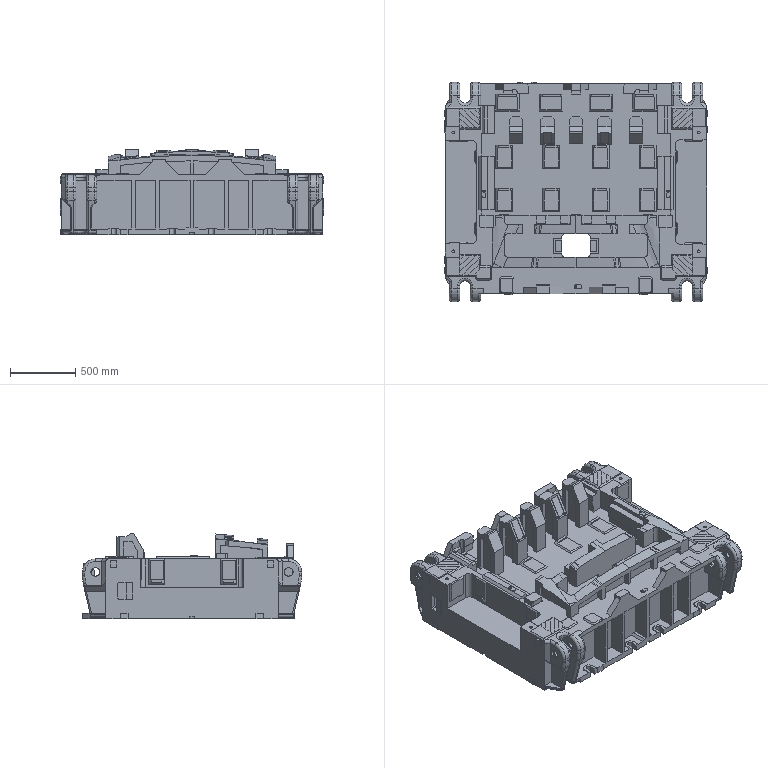Part | NX | features solid 2 | 1 solid | 1661 faces | box 2020 x 1680 x 657.116 mm | volume 538291554 mm3 | plane 1264 | cylinder 277 | spline 46 | torus 40 | cone 26 | sphere 8 | commonest cylinder face diameters 40 x89 68 x48 20 x47 80 x36 64 x16 60 x10